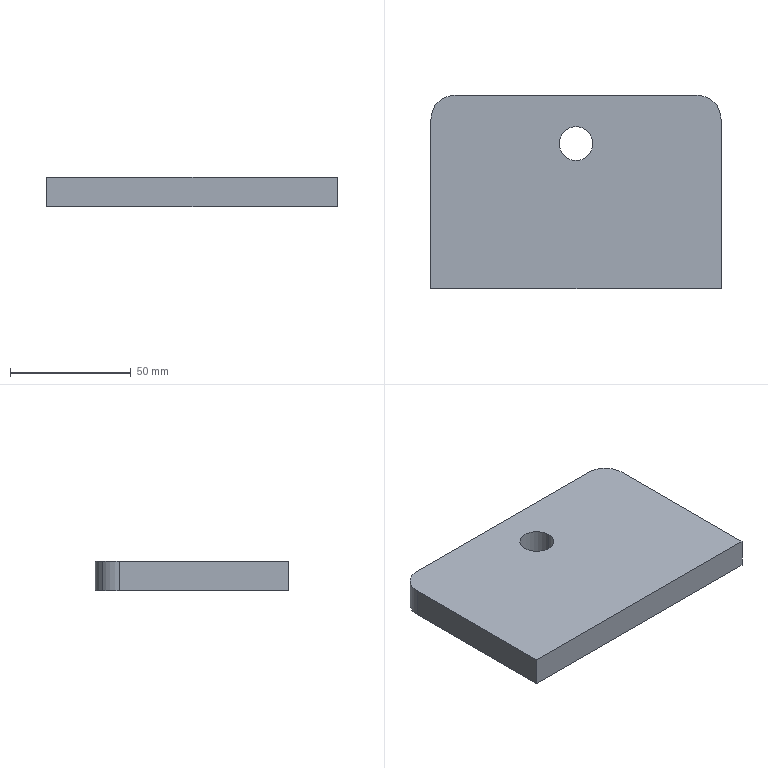Part | STEP file | DCV-000-022 | 1 solid | 12 faces | box 120 x 80 x 12 mm | volume 112838 mm3 | cylinder 6 | plane 6 | commonest cylinder face diameters 20 x4 14 x2
STEP:
#1=CARTESIAN_POINT('',(0.,0.,0.));
#2=DIRECTION('',(0.,0.,1.));
#3=DIRECTION('',(1.,0.,0.));
#4=AXIS2_PLACEMENT_3D('',#1,#2,#3);
#5=CARTESIAN_POINT('',(60.,70.,0.));
#6=VERTEX_POINT('',#5);
#7=CARTESIAN_POINT('',(57.071,77.071,0.));
#8=VERTEX_POINT('',#7);
#9=CARTESIAN_POINT('',(50.,70.,0.));
#10=DIRECTION('',(0.,0.,1.));
#11=DIRECTION('',(0.7071,0.7071,0.));
#12=AXIS2_PLACEMENT_3D('',#9,#10,#11);
#13=CIRCLE('',#12,10.);
#14=CARTESIAN_POINT('',(50.,70.,0.));
#15=DIRECTION('',(0.,0.,1.));
#16=DIRECTION('',(0.7071,0.7071,0.));
#17=AXIS2_PLACEMENT_3D('',#14,#15,#16);
#18=CYLINDRICAL_SURFACE('',#17,10.);
#19=CARTESIAN_POINT('',(0.,0.));
#20=DIRECTION('',(1.,0.));
#21=VECTOR('',#20,1.);
#22=LINE('',#19,#21);
#23=(GEOMETRIC_REPRESENTATION_CONTEXT(2)PARAMETRIC_REPRESENTATION_CONTEXT()REPRESENTATION_CONTEXT('',''));
#24=DEFINITIONAL_REPRESENTATION('',(#22),#23);
#25=PCURVE('',#18,#24);
#26=CARTESIAN_POINT('',(-0.000004309,40.,0.));
#27=DIRECTION('',(0.,0.,1.));
#28=DIRECTION('',(1.,0.,0.));
#29=AXIS2_PLACEMENT_3D('',#26,#27,#28);
#30=PLANE('',#29);
#31=CARTESIAN_POINT('',(50.,30.));
#32=DIRECTION('',(0.7071,0.7071));
#33=AXIS2_PLACEMENT_2D('',#31,#32);
#34=CIRCLE('',#33,10.);
#35=(GEOMETRIC_REPRESENTATION_CONTEXT(2)PARAMETRIC_REPRESENTATION_CONTEXT()REPRESENTATION_CONTEXT('',''));
#36=DEFINITIONAL_REPRESENTATION('',(#34),#35);
#37=PCURVE('',#30,#36);
#38=SURFACE_CURVE('',#13,(#25,#37),.PCURVE_S1.);
#39=EDGE_CURVE('',#6,#8,#38,.T.);
#40=ORIENTED_EDGE('',*,*,#39,.T.);
#41=CARTESIAN_POINT('',(57.071,77.071,12.));
#42=VERTEX_POINT('',#41);
#43=CARTESIAN_POINT('',(57.071,77.071,0.));
#44=DIRECTION('',(0.,0.,1.));
#45=VECTOR('',#44,1.);
#46=LINE('',#43,#45);
#47=CARTESIAN_POINT('',(6.283,0.));
#48=DIRECTION('',(0.,1.));
#49=VECTOR('',#48,1.);
#50=LINE('',#47,#49);
#51=(GEOMETRIC_REPRESENTATION_CONTEXT(2)PARAMETRIC_REPRESENTATION_CONTEXT()REPRESENTATION_CONTEXT('',''));
#52=DEFINITIONAL_REPRESENTATION('',(#50),#51);
#53=PCURVE('',#18,#52);
#54=CARTESIAN_POINT('',(50.,70.,0.));
#55=DIRECTION('',(0.,0.,1.));
#56=DIRECTION('',(0.7071,0.7071,0.));
#57=AXIS2_PLACEMENT_3D('',#54,#55,#56);
#58=CYLINDRICAL_SURFACE('',#57,10.);
#59=CARTESIAN_POINT('',(0.,0.));
#60=DIRECTION('',(0.,1.));
#61=VECTOR('',#60,1.);
#62=LINE('',#59,#61);
#63=(GEOMETRIC_REPRESENTATION_CONTEXT(2)PARAMETRIC_REPRESENTATION_CONTEXT()REPRESENTATION_CONTEXT('',''));
#64=DEFINITIONAL_REPRESENTATION('',(#62),#63);
#65=PCURVE('',#58,#64);
#66=SURFACE_CURVE('',#46,(#53,#65),.PCURVE_S1.);
#67=EDGE_CURVE('',#8,#42,#66,.T.);
#68=ORIENTED_EDGE('',*,*,#67,.T.);
#69=CARTESIAN_POINT('',(60.,70.,12.));
#70=VERTEX_POINT('',#69);
#71=CARTESIAN_POINT('',(50.,70.,12.));
#72=DIRECTION('',(0.,0.,-1.));
#73=DIRECTION('',(0.7071,0.7071,0.));
#74=AXIS2_PLACEMENT_3D('',#71,#72,#73);
#75=CIRCLE('',#74,10.);
#76=CARTESIAN_POINT('',(6.283,12.));
#77=DIRECTION('',(-1.,0.));
#78=VECTOR('',#77,1.);
#79=LINE('',#76,#78);
#80=(GEOMETRIC_REPRESENTATION_CONTEXT(2)PARAMETRIC_REPRESENTATION_CONTEXT()REPRESENTATION_CONTEXT('',''));
#81=DEFINITIONAL_REPRESENTATION('',(#79),#80);
#82=PCURVE('',#18,#81);
#83=CARTESIAN_POINT('',(-0.000004309,40.,12.));
#84=DIRECTION('',(0.,0.,1.));
#85=DIRECTION('',(1.,0.,0.));
#86=AXIS2_PLACEMENT_3D('',#83,#84,#85);
#87=PLANE('',#86);
#88=CARTESIAN_POINT('',(57.071,37.071));
#89=CARTESIAN_POINT('',(69.319,24.824));
#90=CARTESIAN_POINT('',(52.588,20.341));
#91=CARTESIAN_POINT('',(35.858,15.858));
#92=CARTESIAN_POINT('',(40.341,32.588));
#93=CARTESIAN_POINT('',(44.824,49.318));
#94=CARTESIAN_POINT('',(57.071,37.071));
#95=(BOUNDED_CURVE()B_SPLINE_CURVE(2,(#88,#89,#90,#91,#92,#93,#94),.UNSPECIFIED.,.T.,.F.)B_SPLINE_CURVE_WITH_KNOTS((1,2,2,2,2,1),(-2.094,0.,2.094,4.189,6.283,8.378),.UNSPECIFIED.)CURVE()GEOMETRIC_REPRESENTATION_ITEM()RATIONAL_B_SPLINE_CURVE((1.,0.5,1.,0.5,1.,0.5,1.))REPRESENTATION_ITEM(''));
#96=(GEOMETRIC_REPRESENTATION_CONTEXT(2)PARAMETRIC_REPRESENTATION_CONTEXT()REPRESENTATION_CONTEXT('',''));
#97=DEFINITIONAL_REPRESENTATION('',(#95),#96);
#98=PCURVE('',#87,#97);
#99=SURFACE_CURVE('',#75,(#82,#98),.PCURVE_S1.);
#100=EDGE_CURVE('',#42,#70,#99,.T.);
#101=ORIENTED_EDGE('',*,*,#100,.T.);
#102=CARTESIAN_POINT('',(60.,70.,0.));
#103=DIRECTION('',(0.,0.,-1.));
#104=VECTOR('',#103,1.);
#105=LINE('',#102,#104);
#106=CARTESIAN_POINT('',(5.498,0.));
#107=DIRECTION('',(0.,-1.));
#108=VECTOR('',#107,1.);
#109=LINE('',#106,#108);
#110=(GEOMETRIC_REPRESENTATION_CONTEXT(2)PARAMETRIC_REPRESENTATION_CONTEXT()REPRESENTATION_CONTEXT('',''));
#111=DEFINITIONAL_REPRESENTATION('',(#109),#110);
#112=PCURVE('',#18,#111);
#113=CARTESIAN_POINT('',(60.,-0.000000612,0.));
#114=DIRECTION('',(1.,-0.000000215,0.));
#115=DIRECTION('',(0.,0.,-1.));
#116=AXIS2_PLACEMENT_3D('',#113,#114,#115);
#117=PLANE('',#116);
#118=CARTESIAN_POINT('',(0.,70.));
#119=DIRECTION('',(1.,0.));
#120=VECTOR('',#119,1.);
#121=LINE('',#118,#120);
#122=(GEOMETRIC_REPRESENTATION_CONTEXT(2)PARAMETRIC_REPRESENTATION_CONTEXT()REPRESENTATION_CONTEXT('',''));
#123=DEFINITIONAL_REPRESENTATION('',(#121),#122);
#124=PCURVE('',#117,#123);
#125=SURFACE_CURVE('',#105,(#112,#124),.PCURVE_S1.);
#126=EDGE_CURVE('',#70,#6,#125,.T.);
#127=ORIENTED_EDGE('',*,*,#126,.T.);
#128=EDGE_LOOP('',(#40,#68,#101,#127));
#129=FACE_BOUND('',#128,.T.);
#130=ADVANCED_FACE('',(#129),#18,.T.);
#131=CARTESIAN_POINT('',(-50.,80.,0.));
#132=VERTEX_POINT('',#131);
#133=CARTESIAN_POINT('',(-57.071,77.071,0.));
#134=VERTEX_POINT('',#133);
#135=CARTESIAN_POINT('',(-50.,70.,0.));
#136=DIRECTION('',(0.,0.,1.));
#137=DIRECTION('',(-0.7071,0.7071,0.));
#138=AXIS2_PLACEMENT_3D('',#135,#136,#137);
#139=CIRCLE('',#138,10.);
#140=CARTESIAN_POINT('',(-50.,70.,0.));
#141=DIRECTION('',(0.,0.,1.));
#142=DIRECTION('',(-0.7071,0.7071,0.));
#143=AXIS2_PLACEMENT_3D('',#140,#141,#142);
#144=CYLINDRICAL_SURFACE('',#143,10.);
#145=CARTESIAN_POINT('',(0.,0.));
#146=DIRECTION('',(1.,0.));
#147=VECTOR('',#146,1.);
#148=LINE('',#145,#147);
#149=(GEOMETRIC_REPRESENTATION_CONTEXT(2)PARAMETRIC_REPRESENTATION_CONTEXT()REPRESENTATION_CONTEXT('',''));
#150=DEFINITIONAL_REPRESENTATION('',(#148),#149);
#151=PCURVE('',#144,#150);
#152=CARTESIAN_POINT('',(-50.,30.));
#153=DIRECTION('',(-0.7071,0.7071));
#154=AXIS2_PLACEMENT_2D('',#152,#153);
#155=CIRCLE('',#154,10.);
#156=(GEOMETRIC_REPRESENTATION_CONTEXT(2)PARAMETRIC_REPRESENTATION_CONTEXT()REPRESENTATION_CONTEXT('',''));
#157=DEFINITIONAL_REPRESENTATION('',(#155),#156);
#158=PCURVE('',#30,#157);
#159=SURFACE_CURVE('',#139,(#151,#158),.PCURVE_S1.);
#160=EDGE_CURVE('',#132,#134,#159,.T.);
#161=ORIENTED_EDGE('',*,*,#160,.T.);
#162=CARTESIAN_POINT('',(-57.071,77.071,12.));
#163=VERTEX_POINT('',#162);
#164=CARTESIAN_POINT('',(-57.071,77.071,0.));
#165=DIRECTION('',(0.,0.,1.));
#166=VECTOR('',#165,1.);
#167=LINE('',#164,#166);
#168=CARTESIAN_POINT('',(6.283,0.));
#169=DIRECTION('',(0.,1.));
#170=VECTOR('',#169,1.);
#171=LINE('',#168,#170);
#172=(GEOMETRIC_REPRESENTATION_CONTEXT(2)PARAMETRIC_REPRESENTATION_CONTEXT()REPRESENTATION_CONTEXT('',''));
#173=DEFINITIONAL_REPRESENTATION('',(#171),#172);
#174=PCURVE('',#144,#173);
#175=CARTESIAN_POINT('',(-50.,70.,0.));
#176=DIRECTION('',(0.,0.,1.));
#177=DIRECTION('',(-0.7071,0.7071,0.));
#178=AXIS2_PLACEMENT_3D('',#175,#176,#177);
#179=CYLINDRICAL_SURFACE('',#178,10.);
#180=CARTESIAN_POINT('',(0.,0.));
#181=DIRECTION('',(0.,1.));
#182=VECTOR('',#181,1.);
#183=LINE('',#180,#182);
#184=(GEOMETRIC_REPRESENTATION_CONTEXT(2)PARAMETRIC_REPRESENTATION_CONTEXT()REPRESENTATION_CONTEXT('',''));
#185=DEFINITIONAL_REPRESENTATION('',(#183),#184);
#186=PCURVE('',#179,#185);
#187=SURFACE_CURVE('',#167,(#174,#186),.PCURVE_S1.);
#188=EDGE_CURVE('',#134,#163,#187,.T.);
#189=ORIENTED_EDGE('',*,*,#188,.T.);
#190=CARTESIAN_POINT('',(-50.,80.,12.));
#191=VERTEX_POINT('',#190);
#192=CARTESIAN_POINT('',(-50.,70.,12.));
#193=DIRECTION('',(0.,0.,-1.));
#194=DIRECTION('',(-0.7071,0.7071,0.));
#195=AXIS2_PLACEMENT_3D('',#192,#193,#194);
#196=CIRCLE('',#195,10.);
#197=CARTESIAN_POINT('',(6.283,12.));
#198=DIRECTION('',(-1.,0.));
#199=VECTOR('',#198,1.);
#200=LINE('',#197,#199);
#201=(GEOMETRIC_REPRESENTATION_CONTEXT(2)PARAMETRIC_REPRESENTATION_CONTEXT()REPRESENTATION_CONTEXT('',''));
#202=DEFINITIONAL_REPRESENTATION('',(#200),#201);
#203=PCURVE('',#144,#202);
#204=CARTESIAN_POINT('',(-57.071,37.071));
#205=CARTESIAN_POINT('',(-44.824,49.319));
#206=CARTESIAN_POINT('',(-40.341,32.588));
#207=CARTESIAN_POINT('',(-35.858,15.858));
#208=CARTESIAN_POINT('',(-52.588,20.341));
#209=CARTESIAN_POINT('',(-69.319,24.824));
#210=CARTESIAN_POINT('',(-57.071,37.071));
#211=(BOUNDED_CURVE()B_SPLINE_CURVE(2,(#204,#205,#206,#207,#208,#209,#210),.UNSPECIFIED.,.T.,.F.)B_SPLINE_CURVE_WITH_KNOTS((1,2,2,2,2,1),(-2.094,0.,2.094,4.189,6.283,8.378),.UNSPECIFIED.)CURVE()GEOMETRIC_REPRESENTATION_ITEM()RATIONAL_B_SPLINE_CURVE((1.,0.5,1.,0.5,1.,0.5,1.))REPRESENTATION_ITEM(''));
#212=(GEOMETRIC_REPRESENTATION_CONTEXT(2)PARAMETRIC_REPRESENTATION_CONTEXT()REPRESENTATION_CONTEXT('',''));
#213=DEFINITIONAL_REPRESENTATION('',(#211),#212);
#214=PCURVE('',#87,#213);
#215=SURFACE_CURVE('',#196,(#203,#214),.PCURVE_S1.);
#216=EDGE_CURVE('',#163,#191,#215,.T.);
#217=ORIENTED_EDGE('',*,*,#216,.T.);
#218=CARTESIAN_POINT('',(-50.,80.,0.));
#219=DIRECTION('',(0.,0.,-1.));
#220=VECTOR('',#219,1.);
#221=LINE('',#218,#220);
#222=CARTESIAN_POINT('',(5.498,0.));
#223=DIRECTION('',(0.,-1.));
#224=VECTOR('',#223,1.);
#225=LINE('',#222,#224);
#226=(GEOMETRIC_REPRESENTATION_CONTEXT(2)PARAMETRIC_REPRESENTATION_CONTEXT()REPRESENTATION_CONTEXT('',''));
#227=DEFINITIONAL_REPRESENTATION('',(#225),#226);
#228=PCURVE('',#144,#227);
#229=CARTESIAN_POINT('',(60.,80.,0.));
#230=DIRECTION('',(0.000000215,1.,0.));
#231=DIRECTION('',(0.,0.,-1.));
#232=AXIS2_PLACEMENT_3D('',#229,#230,#231);
#233=PLANE('',#232);
#234=CARTESIAN_POINT('',(0.,110.));
#235=DIRECTION('',(1.,0.));
#236=VECTOR('',#235,1.);
#237=LINE('',#234,#236);
#238=(GEOMETRIC_REPRESENTATION_CONTEXT(2)PARAMETRIC_REPRESENTATION_CONTEXT()REPRESENTATION_CONTEXT('',''));
#239=DEFINITIONAL_REPRESENTATION('',(#237),#238);
#240=PCURVE('',#233,#239);
#241=SURFACE_CURVE('',#221,(#228,#240),.PCURVE_S1.);
#242=EDGE_CURVE('',#191,#132,#241,.T.);
#243=ORIENTED_EDGE('',*,*,#242,.T.);
#244=EDGE_LOOP('',(#161,#189,#217,#243));
#245=FACE_BOUND('',#244,.T.);
#246=ADVANCED_FACE('',(#245),#144,.T.);
#247=CARTESIAN_POINT('',(7.,60.,0.));
#248=VERTEX_POINT('',#247);
#249=CARTESIAN_POINT('',(7.,60.,12.));
#250=VERTEX_POINT('',#249);
#251=CARTESIAN_POINT('',(7.,60.,144.72));
#252=DIRECTION('',(0.,0.,1.));
#253=VECTOR('',#252,1.);
#254=LINE('',#251,#253);
#255=CARTESIAN_POINT('',(0.,60.,144.72));
#256=DIRECTION('',(0.,0.,1.));
#257=DIRECTION('',(1.,0.,0.));
#258=AXIS2_PLACEMENT_3D('',#255,#256,#257);
#259=CYLINDRICAL_SURFACE('',#258,7.);
#260=CARTESIAN_POINT('',(6.283,0.));
#261=DIRECTION('',(0.,1.));
#262=VECTOR('',#261,1.);
#263=LINE('',#260,#262);
#264=(GEOMETRIC_REPRESENTATION_CONTEXT(2)PARAMETRIC_REPRESENTATION_CONTEXT()REPRESENTATION_CONTEXT('',''));
#265=DEFINITIONAL_REPRESENTATION('',(#263),#264);
#266=PCURVE('',#259,#265);
#267=CARTESIAN_POINT('',(0.,60.,144.72));
#268=DIRECTION('',(0.,0.,1.));
#269=DIRECTION('',(1.,0.,0.));
#270=AXIS2_PLACEMENT_3D('',#267,#268,#269);
#271=CYLINDRICAL_SURFACE('',#270,7.);
#272=CARTESIAN_POINT('',(0.,0.));
#273=DIRECTION('',(0.,1.));
#274=VECTOR('',#273,1.);
#275=LINE('',#272,#274);
#276=(GEOMETRIC_REPRESENTATION_CONTEXT(2)PARAMETRIC_REPRESENTATION_CONTEXT()REPRESENTATION_CONTEXT('',''));
#277=DEFINITIONAL_REPRESENTATION('',(#275),#276);
#278=PCURVE('',#271,#277);
#279=SURFACE_CURVE('',#254,(#266,#278),.PCURVE_S1.);
#280=EDGE_CURVE('',#248,#250,#279,.T.);
#281=ORIENTED_EDGE('',*,*,#280,.T.);
#282=CARTESIAN_POINT('',(-7.,60.,12.));
#283=VERTEX_POINT('',#282);
#284=CARTESIAN_POINT('',(0.,60.,12.));
#285=DIRECTION('',(0.,0.,-1.));
#286=DIRECTION('',(1.,0.,0.));
#287=AXIS2_PLACEMENT_3D('',#284,#285,#286);
#288=CIRCLE('',#287,7.);
#289=CARTESIAN_POINT('',(6.283,-132.72));
#290=DIRECTION('',(-1.,0.));
#291=VECTOR('',#290,1.);
#292=LINE('',#289,#291);
#293=(GEOMETRIC_REPRESENTATION_CONTEXT(2)PARAMETRIC_REPRESENTATION_CONTEXT()REPRESENTATION_CONTEXT('',''));
#294=DEFINITIONAL_REPRESENTATION('',(#292),#293);
#295=PCURVE('',#259,#294);
#296=CARTESIAN_POINT('',(7.,20.));
#297=CARTESIAN_POINT('',(7.,7.876));
#298=CARTESIAN_POINT('',(-3.5,13.938));
#299=CARTESIAN_POINT('',(-14.,20.));
#300=CARTESIAN_POINT('',(-3.5,26.062));
#301=CARTESIAN_POINT('',(7.,32.124));
#302=CARTESIAN_POINT('',(7.,20.));
#303=(BOUNDED_CURVE()B_SPLINE_CURVE(2,(#296,#297,#298,#299,#300,#301,#302),.UNSPECIFIED.,.T.,.F.)B_SPLINE_CURVE_WITH_KNOTS((1,2,2,2,2,1),(-2.094,0.,2.094,4.189,6.283,8.378),.UNSPECIFIED.)CURVE()GEOMETRIC_REPRESENTATION_ITEM()RATIONAL_B_SPLINE_CURVE((1.,0.5,1.,0.5,1.,0.5,1.))REPRESENTATION_ITEM(''));
#304=(GEOMETRIC_REPRESENTATION_CONTEXT(2)PARAMETRIC_REPRESENTATION_CONTEXT()REPRESENTATION_CONTEXT('',''));
#305=DEFINITIONAL_REPRESENTATION('',(#303),#304);
#306=PCURVE('',#87,#305);
#307=SURFACE_CURVE('',#288,(#295,#306),.PCURVE_S1.);
#308=EDGE_CURVE('',#250,#283,#307,.T.);
#309=ORIENTED_EDGE('',*,*,#308,.T.);
#310=CARTESIAN_POINT('',(-7.,60.,0.));
#311=VERTEX_POINT('',#310);
#312=CARTESIAN_POINT('',(-7.,60.,144.72));
#313=DIRECTION('',(0.,0.,1.));
#314=VECTOR('',#313,1.);
#315=LINE('',#312,#314);
#316=CARTESIAN_POINT('',(3.142,0.));
#317=DIRECTION('',(0.,1.));
#318=VECTOR('',#317,1.);
#319=LINE('',#316,#318);
#320=(GEOMETRIC_REPRESENTATION_CONTEXT(2)PARAMETRIC_REPRESENTATION_CONTEXT()REPRESENTATION_CONTEXT('',''));
#321=DEFINITIONAL_REPRESENTATION('',(#319),#320);
#322=PCURVE('',#259,#321);
#323=CARTESIAN_POINT('',(3.142,0.));
#324=DIRECTION('',(0.,1.));
#325=VECTOR('',#324,1.);
#326=LINE('',#323,#325);
#327=(GEOMETRIC_REPRESENTATION_CONTEXT(2)PARAMETRIC_REPRESENTATION_CONTEXT()REPRESENTATION_CONTEXT('',''));
#328=DEFINITIONAL_REPRESENTATION('',(#326),#327);
#329=PCURVE('',#271,#328);
#330=SURFACE_CURVE('',#315,(#322,#329),.PCURVE_S1.);
#331=EDGE_CURVE('',#311,#283,#330,.T.);
#332=ORIENTED_EDGE('',*,*,#331,.F.);
#333=CARTESIAN_POINT('',(0.,60.,0.));
#334=DIRECTION('',(0.,0.,1.));
#335=DIRECTION('',(1.,0.,0.));
#336=AXIS2_PLACEMENT_3D('',#333,#334,#335);
#337=CIRCLE('',#336,7.);
#338=CARTESIAN_POINT('',(0.,-144.72));
#339=DIRECTION('',(1.,0.));
#340=VECTOR('',#339,1.);
#341=LINE('',#338,#340);
#342=(GEOMETRIC_REPRESENTATION_CONTEXT(2)PARAMETRIC_REPRESENTATION_CONTEXT()REPRESENTATION_CONTEXT('',''));
#343=DEFINITIONAL_REPRESENTATION('',(#341),#342);
#344=PCURVE('',#259,#343);
#345=CARTESIAN_POINT('',(0.000004309,20.));
#346=DIRECTION('',(1.,0.));
#347=AXIS2_PLACEMENT_2D('',#345,#346);
#348=CIRCLE('',#347,7.);
#349=(GEOMETRIC_REPRESENTATION_CONTEXT(2)PARAMETRIC_REPRESENTATION_CONTEXT()REPRESENTATION_CONTEXT('',''));
#350=DEFINITIONAL_REPRESENTATION('',(#348),#349);
#351=PCURVE('',#30,#350);
#352=SURFACE_CURVE('',#337,(#344,#351),.PCURVE_S1.);
#353=EDGE_CURVE('',#311,#248,#352,.T.);
#354=ORIENTED_EDGE('',*,*,#353,.T.);
#355=EDGE_LOOP('',(#281,#309,#332,#354));
#356=FACE_BOUND('',#355,.F.);
#357=ADVANCED_FACE('',(#356),#259,.F.);
#358=ORIENTED_EDGE('',*,*,#308,.T.);
#359=CARTESIAN_POINT('',(0.,60.,12.));
#360=DIRECTION('',(0.,0.,-1.));
#361=DIRECTION('',(1.,0.,0.));
#362=AXIS2_PLACEMENT_3D('',#359,#360,#361);
#363=CIRCLE('',#362,7.);
#364=CARTESIAN_POINT('',(7.,20.));
#365=CARTESIAN_POINT('',(7.,7.876));
#366=CARTESIAN_POINT('',(-3.5,13.938));
#367=CARTESIAN_POINT('',(-14.,20.));
#368=CARTESIAN_POINT('',(-3.5,26.062));
#369=CARTESIAN_POINT('',(7.,32.124));
#370=CARTESIAN_POINT('',(7.,20.));
#371=(BOUNDED_CURVE()B_SPLINE_CURVE(2,(#364,#365,#366,#367,#368,#369,#370),.UNSPECIFIED.,.T.,.F.)B_SPLINE_CURVE_WITH_KNOTS((1,2,2,2,2,1),(-2.094,0.,2.094,4.189,6.283,8.378),.UNSPECIFIED.)CURVE()GEOMETRIC_REPRESENTATION_ITEM()RATIONAL_B_SPLINE_CURVE((1.,0.5,1.,0.5,1.,0.5,1.))REPRESENTATION_ITEM(''));
#372=(GEOMETRIC_REPRESENTATION_CONTEXT(2)PARAMETRIC_REPRESENTATION_CONTEXT()REPRESENTATION_CONTEXT('',''));
#373=DEFINITIONAL_REPRESENTATION('',(#371),#372);
#374=PCURVE('',#87,#373);
#375=CARTESIAN_POINT('',(6.283,-132.72));
#376=DIRECTION('',(-1.,0.));
#377=VECTOR('',#376,1.);
#378=LINE('',#375,#377);
#379=(GEOMETRIC_REPRESENTATION_CONTEXT(2)PARAMETRIC_REPRESENTATION_CONTEXT()REPRESENTATION_CONTEXT('',''));
#380=DEFINITIONAL_REPRESENTATION('',(#378),#379);
#381=PCURVE('',#271,#380);
#382=SURFACE_CURVE('',#363,(#374,#381),.PCURVE_S1.);
#383=EDGE_CURVE('',#283,#250,#382,.T.);
#384=ORIENTED_EDGE('',*,*,#383,.T.);
#385=EDGE_LOOP('',(#358,#384));
#386=FACE_BOUND('',#385,.T.);
#387=CARTESIAN_POINT('',(50.,80.,12.));
#388=VERTEX_POINT('',#387);
#389=CARTESIAN_POINT('',(50.,70.,12.));
#390=DIRECTION('',(0.,0.,-1.));
#391=DIRECTION('',(0.7071,0.7071,0.));
#392=AXIS2_PLACEMENT_3D('',#389,#390,#391);
#393=CIRCLE('',#392,10.);
#394=CARTESIAN_POINT('',(57.071,37.071));
#395=CARTESIAN_POINT('',(69.319,24.824));
#396=CARTESIAN_POINT('',(52.588,20.341));
#397=CARTESIAN_POINT('',(35.858,15.858));
#398=CARTESIAN_POINT('',(40.341,32.588));
#399=CARTESIAN_POINT('',(44.824,49.318));
#400=CARTESIAN_POINT('',(57.071,37.071));
#401=(BOUNDED_CURVE()B_SPLINE_CURVE(2,(#394,#395,#396,#397,#398,#399,#400),.UNSPECIFIED.,.T.,.F.)B_SPLINE_CURVE_WITH_KNOTS((1,2,2,2,2,1),(-2.094,0.,2.094,4.189,6.283,8.378),.UNSPECIFIED.)CURVE()GEOMETRIC_REPRESENTATION_ITEM()RATIONAL_B_SPLINE_CURVE((1.,0.5,1.,0.5,1.,0.5,1.))REPRESENTATION_ITEM(''));
#402=(GEOMETRIC_REPRESENTATION_CONTEXT(2)PARAMETRIC_REPRESENTATION_CONTEXT()REPRESENTATION_CONTEXT('',''));
#403=DEFINITIONAL_REPRESENTATION('',(#401),#402);
#404=PCURVE('',#87,#403);
#405=CARTESIAN_POINT('',(6.283,12.));
#406=DIRECTION('',(-1.,0.));
#407=VECTOR('',#406,1.);
#408=LINE('',#405,#407);
#409=(GEOMETRIC_REPRESENTATION_CONTEXT(2)PARAMETRIC_REPRESENTATION_CONTEXT()REPRESENTATION_CONTEXT('',''));
#410=DEFINITIONAL_REPRESENTATION('',(#408),#409);
#411=PCURVE('',#58,#410);
#412=SURFACE_CURVE('',#393,(#404,#411),.PCURVE_S1.);
#413=EDGE_CURVE('',#388,#42,#412,.T.);
#414=ORIENTED_EDGE('',*,*,#413,.F.);
#415=CARTESIAN_POINT('',(60.,80.,12.));
#416=DIRECTION('',(-1.,0.000000215,0.));
#417=VECTOR('',#416,1.);
#418=LINE('',#415,#417);
#419=CARTESIAN_POINT('',(60.,40.));
#420=DIRECTION('',(-1.,0.000000215));
#421=VECTOR('',#420,1.);
#422=LINE('',#419,#421);
#423=(GEOMETRIC_REPRESENTATION_CONTEXT(2)PARAMETRIC_REPRESENTATION_CONTEXT()REPRESENTATION_CONTEXT('',''));
#424=DEFINITIONAL_REPRESENTATION('',(#422),#423);
#425=PCURVE('',#87,#424);
#426=CARTESIAN_POINT('',(-12.,0.));
#427=DIRECTION('',(0.,1.));
#428=VECTOR('',#427,1.);
#429=LINE('',#426,#428);
#430=(GEOMETRIC_REPRESENTATION_CONTEXT(2)PARAMETRIC_REPRESENTATION_CONTEXT()REPRESENTATION_CONTEXT('',''));
#431=DEFINITIONAL_REPRESENTATION('',(#429),#430);
#432=PCURVE('',#233,#431);
#433=SURFACE_CURVE('',#418,(#425,#432),.PCURVE_S1.);
#434=EDGE_CURVE('',#388,#191,#433,.T.);
#435=ORIENTED_EDGE('',*,*,#434,.T.);
#436=ORIENTED_EDGE('',*,*,#216,.F.);
#437=CARTESIAN_POINT('',(-60.,70.,12.));
#438=VERTEX_POINT('',#437);
#439=CARTESIAN_POINT('',(-50.,70.,12.));
#440=DIRECTION('',(0.,0.,-1.));
#441=DIRECTION('',(-0.7071,0.7071,0.));
#442=AXIS2_PLACEMENT_3D('',#439,#440,#441);
#443=CIRCLE('',#442,10.);
#444=CARTESIAN_POINT('',(-57.071,37.071));
#445=CARTESIAN_POINT('',(-44.824,49.319));
#446=CARTESIAN_POINT('',(-40.341,32.588));
#447=CARTESIAN_POINT('',(-35.858,15.858));
#448=CARTESIAN_POINT('',(-52.588,20.341));
#449=CARTESIAN_POINT('',(-69.319,24.824));
#450=CARTESIAN_POINT('',(-57.071,37.071));
#451=(BOUNDED_CURVE()B_SPLINE_CURVE(2,(#444,#445,#446,#447,#448,#449,#450),.UNSPECIFIED.,.T.,.F.)B_SPLINE_CURVE_WITH_KNOTS((1,2,2,2,2,1),(-2.094,0.,2.094,4.189,6.283,8.378),.UNSPECIFIED.)CURVE()GEOMETRIC_REPRESENTATION_ITEM()RATIONAL_B_SPLINE_CURVE((1.,0.5,1.,0.5,1.,0.5,1.))REPRESENTATION_ITEM(''));
#452=(GEOMETRIC_REPRESENTATION_CONTEXT(2)PARAMETRIC_REPRESENTATION_CONTEXT()REPRESENTATION_CONTEXT('',''));
#453=DEFINITIONAL_REPRESENTATION('',(#451),#452);
#454=PCURVE('',#87,#453);
#455=CARTESIAN_POINT('',(6.283,12.));
#456=DIRECTION('',(-1.,0.));
#457=VECTOR('',#456,1.);
#458=LINE('',#455,#457);
#459=(GEOMETRIC_REPRESENTATION_CONTEXT(2)PARAMETRIC_REPRESENTATION_CONTEXT()REPRESENTATION_CONTEXT('',''));
#460=DEFINITIONAL_REPRESENTATION('',(#458),#459);
#461=PCURVE('',#179,#460);
#462=SURFACE_CURVE('',#443,(#454,#461),.PCURVE_S1.);
#463=EDGE_CURVE('',#438,#163,#462,.T.);
#464=ORIENTED_EDGE('',*,*,#463,.F.);
#465=CARTESIAN_POINT('',(-60.,0.000000612,12.));
#466=VERTEX_POINT('',#465);
#467=CARTESIAN_POINT('',(-60.,80.,12.));
#468=DIRECTION('',(-0.000000215,-1.,0.));
#469=VECTOR('',#468,1.);
#470=LINE('',#467,#469);
#471=CARTESIAN_POINT('',(-60.,40.));
#472=DIRECTION('',(-0.000000215,-1.));
#473=VECTOR('',#472,1.);
#474=LINE('',#471,#473);
#475=(GEOMETRIC_REPRESENTATION_CONTEXT(2)PARAMETRIC_REPRESENTATION_CONTEXT()REPRESENTATION_CONTEXT('',''));
#476=DEFINITIONAL_REPRESENTATION('',(#474),#475);
#477=PCURVE('',#87,#476);
#478=CARTESIAN_POINT('',(-60.,80.,0.));
#479=DIRECTION('',(-1.,0.000000215,0.));
#480=DIRECTION('',(0.,0.,1.));
#481=AXIS2_PLACEMENT_3D('',#478,#479,#480);
#482=PLANE('',#481);
#483=CARTESIAN_POINT('',(12.,0.));
#484=DIRECTION('',(0.,-1.));
#485=VECTOR('',#484,1.);
#486=LINE('',#483,#485);
#487=(GEOMETRIC_REPRESENTATION_CONTEXT(2)PARAMETRIC_REPRESENTATION_CONTEXT()REPRESENTATION_CONTEXT('',''));
#488=DEFINITIONAL_REPRESENTATION('',(#486),#487);
#489=PCURVE('',#482,#488);
#490=SURFACE_CURVE('',#470,(#477,#489),.PCURVE_S1.);
#491=EDGE_CURVE('',#438,#466,#490,.T.);
#492=ORIENTED_EDGE('',*,*,#491,.T.);
#493=CARTESIAN_POINT('',(60.,-0.000000612,12.));
#494=VERTEX_POINT('',#493);
#495=CARTESIAN_POINT('',(-60.,0.000000612,12.));
#496=DIRECTION('',(1.,-0.00000001,0.));
#497=VECTOR('',#496,1.);
#498=LINE('',#495,#497);
#499=CARTESIAN_POINT('',(-60.,-40.));
#500=DIRECTION('',(1.,-0.00000001));
#501=VECTOR('',#500,1.);
#502=LINE('',#499,#501);
#503=(GEOMETRIC_REPRESENTATION_CONTEXT(2)PARAMETRIC_REPRESENTATION_CONTEXT()REPRESENTATION_CONTEXT('',''));
#504=DEFINITIONAL_REPRESENTATION('',(#502),#503);
#505=PCURVE('',#87,#504);
#506=CARTESIAN_POINT('',(-60.,0.000000612,0.));
#507=DIRECTION('',(-0.00000001,-1.,0.));
#508=DIRECTION('',(-1.,0.00000001,0.));
#509=AXIS2_PLACEMENT_3D('',#506,#507,#508);
#510=PLANE('',#509);
#511=CARTESIAN_POINT('',(0.,-12.));
#512=DIRECTION('',(-1.,0.));
#513=VECTOR('',#512,1.);
#514=LINE('',#511,#513);
#515=(GEOMETRIC_REPRESENTATION_CONTEXT(2)PARAMETRIC_REPRESENTATION_CONTEXT()REPRESENTATION_CONTEXT('',''));
#516=DEFINITIONAL_REPRESENTATION('',(#514),#515);
#517=PCURVE('',#510,#516);
#518=SURFACE_CURVE('',#498,(#505,#517),.PCURVE_S1.);
#519=EDGE_CURVE('',#466,#494,#518,.T.);
#520=ORIENTED_EDGE('',*,*,#519,.T.);
#521=CARTESIAN_POINT('',(60.,-0.000000612,12.));
#522=DIRECTION('',(0.000000215,1.,0.));
#523=VECTOR('',#522,1.);
#524=LINE('',#521,#523);
#525=CARTESIAN_POINT('',(60.,-40.));
#526=DIRECTION('',(0.000000215,1.));
#527=VECTOR('',#526,1.);
#528=LINE('',#525,#527);
#529=(GEOMETRIC_REPRESENTATION_CONTEXT(2)PARAMETRIC_REPRESENTATION_CONTEXT()REPRESENTATION_CONTEXT('',''));
#530=DEFINITIONAL_REPRESENTATION('',(#528),#529);
#531=PCURVE('',#87,#530);
#532=CARTESIAN_POINT('',(-12.,0.));
#533=DIRECTION('',(0.,1.));
#534=VECTOR('',#533,1.);
#535=LINE('',#532,#534);
#536=(GEOMETRIC_REPRESENTATION_CONTEXT(2)PARAMETRIC_REPRESENTATION_CONTEXT()REPRESENTATION_CONTEXT('',''));
#537=DEFINITIONAL_REPRESENTATION('',(#535),#536);
#538=PCURVE('',#117,#537);
#539=SURFACE_CURVE('',#524,(#531,#538),.PCURVE_S1.);
#540=EDGE_CURVE('',#494,#70,#539,.T.);
#541=ORIENTED_EDGE('',*,*,#540,.T.);
#542=ORIENTED_EDGE('',*,*,#100,.F.);
#543=EDGE_LOOP('',(#414,#435,#436,#464,#492,#520,#541,#542));
#544=FACE_BOUND('',#543,.T.);
#545=ADVANCED_FACE('',(#386,#544),#87,.T.);
#546=CARTESIAN_POINT('',(-60.,70.,0.));
#547=VERTEX_POINT('',#546);
#548=CARTESIAN_POINT('',(-60.,70.,0.));
#549=DIRECTION('',(0.,0.,1.));
#550=VECTOR('',#549,1.);
#551=LINE('',#548,#550);
#552=CARTESIAN_POINT('',(0.,-10.));
#553=DIRECTION('',(1.,0.));
#554=VECTOR('',#553,1.);
#555=LINE('',#552,#554);
#556=(GEOMETRIC_REPRESENTATION_CONTEXT(2)PARAMETRIC_REPRESENTATION_CONTEXT()REPRESENTATION_CONTEXT('',''));
#557=DEFINITIONAL_REPRESENTATION('',(#555),#556);
#558=PCURVE('',#482,#557);
#559=CARTESIAN_POINT('',(0.7854,0.));
#560=DIRECTION('',(0.,1.));
#561=VECTOR('',#560,1.);
#562=LINE('',#559,#561);
#563=(GEOMETRIC_REPRESENTATION_CONTEXT(2)PARAMETRIC_REPRESENTATION_CONTEXT()REPRESENTATION_CONTEXT('',''));
#564=DEFINITIONAL_REPRESENTATION('',(#562),#563);
#565=PCURVE('',#179,#564);
#566=SURFACE_CURVE('',#551,(#558,#565),.PCURVE_S1.);
#567=EDGE_CURVE('',#547,#438,#566,.T.);
#568=ORIENTED_EDGE('',*,*,#567,.F.);
#569=CARTESIAN_POINT('',(-60.,0.000000612,0.));
#570=VERTEX_POINT('',#569);
#571=CARTESIAN_POINT('',(-60.,80.,0.));
#572=DIRECTION('',(-0.000000215,-1.,0.));
#573=VECTOR('',#572,1.);
#574=LINE('',#571,#573);
#575=CARTESIAN_POINT('',(0.,0.));
#576=DIRECTION('',(0.,-1.));
#577=VECTOR('',#576,1.);
#578=LINE('',#575,#577);
#579=(GEOMETRIC_REPRESENTATION_CONTEXT(2)PARAMETRIC_REPRESENTATION_CONTEXT()REPRESENTATION_CONTEXT('',''));
#580=DEFINITIONAL_REPRESENTATION('',(#578),#579);
#581=PCURVE('',#482,#580);
#582=CARTESIAN_POINT('',(-60.,40.));
#583=DIRECTION('',(-0.000000215,-1.));
#584=VECTOR('',#583,1.);
#585=LINE('',#582,#584);
#586=(GEOMETRIC_REPRESENTATION_CONTEXT(2)PARAMETRIC_REPRESENTATION_CONTEXT()REPRESENTATION_CONTEXT('',''));
#587=DEFINITIONAL_REPRESENTATION('',(#585),#586);
#588=PCURVE('',#30,#587);
#589=SURFACE_CURVE('',#574,(#581,#588),.PCURVE_S1.);
#590=EDGE_CURVE('',#547,#570,#589,.T.);
#591=ORIENTED_EDGE('',*,*,#590,.T.);
#592=CARTESIAN_POINT('',(-60.,0.000000612,0.));
#593=DIRECTION('',(0.,0.,1.));
#594=VECTOR('',#593,1.);
#595=LINE('',#592,#594);
#596=CARTESIAN_POINT('',(0.,-80.));
#597=DIRECTION('',(1.,0.));
#598=VECTOR('',#597,1.);
#599=LINE('',#596,#598);
#600=(GEOMETRIC_REPRESENTATION_CONTEXT(2)PARAMETRIC_REPRESENTATION_CONTEXT()REPRESENTATION_CONTEXT('',''));
#601=DEFINITIONAL_REPRESENTATION('',(#599),#600);
#602=PCURVE('',#482,#601);
#603=CARTESIAN_POINT('',(0.,0.));
#604=DIRECTION('',(0.,-1.));
#605=VECTOR('',#604,1.);
#606=LINE('',#603,#605);
#607=(GEOMETRIC_REPRESENTATION_CONTEXT(2)PARAMETRIC_REPRESENTATION_CONTEXT()REPRESENTATION_CONTEXT('',''));
#608=DEFINITIONAL_REPRESENTATION('',(#606),#607);
#609=PCURVE('',#510,#608);
#610=SURFACE_CURVE('',#595,(#602,#609),.PCURVE_S1.);
#611=EDGE_CURVE('',#570,#466,#610,.T.);
#612=ORIENTED_EDGE('',*,*,#611,.T.);
#613=ORIENTED_EDGE('',*,*,#491,.F.);
#614=EDGE_LOOP('',(#568,#591,#612,#613));
#615=FACE_BOUND('',#614,.T.);
#616=ADVANCED_FACE('',(#615),#482,.T.);
#617=CARTESIAN_POINT('',(60.,-0.000000612,0.));
#618=VERTEX_POINT('',#617);
#619=CARTESIAN_POINT('',(-60.,0.000000612,0.));
#620=DIRECTION('',(1.,-0.00000001,0.));
#621=VECTOR('',#620,1.);
#622=LINE('',#619,#621);
#623=CARTESIAN_POINT('',(0.,0.));
#624=DIRECTION('',(-1.,0.));
#625=VECTOR('',#624,1.);
#626=LINE('',#623,#625);
#627=(GEOMETRIC_REPRESENTATION_CONTEXT(2)PARAMETRIC_REPRESENTATION_CONTEXT()REPRESENTATION_CONTEXT('',''));
#628=DEFINITIONAL_REPRESENTATION('',(#626),#627);
#629=PCURVE('',#510,#628);
#630=CARTESIAN_POINT('',(-60.,-40.));
#631=DIRECTION('',(1.,-0.00000001));
#632=VECTOR('',#631,1.);
#633=LINE('',#630,#632);
#634=(GEOMETRIC_REPRESENTATION_CONTEXT(2)PARAMETRIC_REPRESENTATION_CONTEXT()REPRESENTATION_CONTEXT('',''));
#635=DEFINITIONAL_REPRESENTATION('',(#633),#634);
#636=PCURVE('',#30,#635);
#637=SURFACE_CURVE('',#622,(#629,#636),.PCURVE_S1.);
#638=EDGE_CURVE('',#570,#618,#637,.T.);
#639=ORIENTED_EDGE('',*,*,#638,.T.);
#640=CARTESIAN_POINT('',(60.,-0.000000612,0.));
#641=DIRECTION('',(0.,0.,1.));
#642=VECTOR('',#641,1.);
#643=LINE('',#640,#642);
#644=CARTESIAN_POINT('',(-120.,0.));
#645=DIRECTION('',(0.,-1.));
#646=VECTOR('',#645,1.);
#647=LINE('',#644,#646);
#648=(GEOMETRIC_REPRESENTATION_CONTEXT(2)PARAMETRIC_REPRESENTATION_CONTEXT()REPRESENTATION_CONTEXT('',''));
#649=DEFINITIONAL_REPRESENTATION('',(#647),#648);
#650=PCURVE('',#510,#649);
#651=CARTESIAN_POINT('',(0.,0.));
#652=DIRECTION('',(-1.,0.));
#653=VECTOR('',#652,1.);
#654=LINE('',#651,#653);
#655=(GEOMETRIC_REPRESENTATION_CONTEXT(2)PARAMETRIC_REPRESENTATION_CONTEXT()REPRESENTATION_CONTEXT('',''));
#656=DEFINITIONAL_REPRESENTATION('',(#654),#655);
#657=PCURVE('',#117,#656);
#658=SURFACE_CURVE('',#643,(#650,#657),.PCURVE_S1.);
#659=EDGE_CURVE('',#618,#494,#658,.T.);
#660=ORIENTED_EDGE('',*,*,#659,.T.);
#661=ORIENTED_EDGE('',*,*,#519,.F.);
#662=ORIENTED_EDGE('',*,*,#611,.F.);
#663=EDGE_LOOP('',(#639,#660,#661,#662));
#664=FACE_BOUND('',#663,.T.);
#665=ADVANCED_FACE('',(#664),#510,.T.);
#666=ORIENTED_EDGE('',*,*,#126,.F.);
#667=ORIENTED_EDGE('',*,*,#540,.F.);
#668=ORIENTED_EDGE('',*,*,#659,.F.);
#669=CARTESIAN_POINT('',(60.,-0.000000612,0.));
#670=DIRECTION('',(0.000000215,1.,0.));
#671=VECTOR('',#670,1.);
#672=LINE('',#669,#671);
#673=CARTESIAN_POINT('',(0.,0.));
#674=DIRECTION('',(0.,1.));
#675=VECTOR('',#674,1.);
#676=LINE('',#673,#675);
#677=(GEOMETRIC_REPRESENTATION_CONTEXT(2)PARAMETRIC_REPRESENTATION_CONTEXT()REPRESENTATION_CONTEXT('',''));
#678=DEFINITIONAL_REPRESENTATION('',(#676),#677);
#679=PCURVE('',#117,#678);
#680=CARTESIAN_POINT('',(60.,-40.));
#681=DIRECTION('',(0.000000215,1.));
#682=VECTOR('',#681,1.);
#683=LINE('',#680,#682);
#684=(GEOMETRIC_REPRESENTATION_CONTEXT(2)PARAMETRIC_REPRESENTATION_CONTEXT()REPRESENTATION_CONTEXT('',''));
#685=DEFINITIONAL_REPRESENTATION('',(#683),#684);
#686=PCURVE('',#30,#685);
#687=SURFACE_CURVE('',#672,(#679,#686),.PCURVE_S1.);
#688=EDGE_CURVE('',#618,#6,#687,.T.);
#689=ORIENTED_EDGE('',*,*,#688,.T.);
#690=EDGE_LOOP('',(#666,#667,#668,#689));
#691=FACE_BOUND('',#690,.T.);
#692=ADVANCED_FACE('',(#691),#117,.T.);
#693=ORIENTED_EDGE('',*,*,#383,.T.);
#694=ORIENTED_EDGE('',*,*,#280,.F.);
#695=CARTESIAN_POINT('',(0.,60.,0.));
#696=DIRECTION('',(0.,0.,1.));
#697=DIRECTION('',(1.,0.,0.));
#698=AXIS2_PLACEMENT_3D('',#695,#696,#697);
#699=CIRCLE('',#698,7.);
#700=CARTESIAN_POINT('',(0.,-144.72));
#701=DIRECTION('',(1.,0.));
#702=VECTOR('',#701,1.);
#703=LINE('',#700,#702);
#704=(GEOMETRIC_REPRESENTATION_CONTEXT(2)PARAMETRIC_REPRESENTATION_CONTEXT()REPRESENTATION_CONTEXT('',''));
#705=DEFINITIONAL_REPRESENTATION('',(#703),#704);
#706=PCURVE('',#271,#705);
#707=CARTESIAN_POINT('',(0.000004309,20.));
#708=DIRECTION('',(1.,0.));
#709=AXIS2_PLACEMENT_2D('',#707,#708);
#710=CIRCLE('',#709,7.);
#711=(GEOMETRIC_REPRESENTATION_CONTEXT(2)PARAMETRIC_REPRESENTATION_CONTEXT()REPRESENTATION_CONTEXT('',''));
#712=DEFINITIONAL_REPRESENTATION('',(#710),#711);
#713=PCURVE('',#30,#712);
#714=SURFACE_CURVE('',#699,(#706,#713),.PCURVE_S1.);
#715=EDGE_CURVE('',#248,#311,#714,.T.);
#716=ORIENTED_EDGE('',*,*,#715,.T.);
#717=ORIENTED_EDGE('',*,*,#331,.T.);
#718=EDGE_LOOP('',(#693,#694,#716,#717));
#719=FACE_BOUND('',#718,.F.);
#720=ADVANCED_FACE('',(#719),#271,.F.);
#721=ORIENTED_EDGE('',*,*,#188,.F.);
#722=CARTESIAN_POINT('',(-50.,70.,0.));
#723=DIRECTION('',(0.,0.,1.));
#724=DIRECTION('',(-0.7071,0.7071,0.));
#725=AXIS2_PLACEMENT_3D('',#722,#723,#724);
#726=CIRCLE('',#725,10.);
#727=CARTESIAN_POINT('',(0.,0.));
#728=DIRECTION('',(1.,0.));
#729=VECTOR('',#728,1.);
#730=LINE('',#727,#729);
#731=(GEOMETRIC_REPRESENTATION_CONTEXT(2)PARAMETRIC_REPRESENTATION_CONTEXT()REPRESENTATION_CONTEXT('',''));
#732=DEFINITIONAL_REPRESENTATION('',(#730),#731);
#733=PCURVE('',#179,#732);
#734=CARTESIAN_POINT('',(-50.,30.));
#735=DIRECTION('',(-0.7071,0.7071));
#736=AXIS2_PLACEMENT_2D('',#734,#735);
#737=CIRCLE('',#736,10.);
#738=(GEOMETRIC_REPRESENTATION_CONTEXT(2)PARAMETRIC_REPRESENTATION_CONTEXT()REPRESENTATION_CONTEXT('',''));
#739=DEFINITIONAL_REPRESENTATION('',(#737),#738);
#740=PCURVE('',#30,#739);
#741=SURFACE_CURVE('',#726,(#733,#740),.PCURVE_S1.);
#742=EDGE_CURVE('',#134,#547,#741,.T.);
#743=ORIENTED_EDGE('',*,*,#742,.T.);
#744=ORIENTED_EDGE('',*,*,#567,.T.);
#745=ORIENTED_EDGE('',*,*,#463,.T.);
#746=EDGE_LOOP('',(#721,#743,#744,#745));
#747=FACE_BOUND('',#746,.T.);
#748=ADVANCED_FACE('',(#747),#179,.T.);
#749=ORIENTED_EDGE('',*,*,#715,.T.);
#750=ORIENTED_EDGE('',*,*,#353,.T.);
#751=EDGE_LOOP('',(#749,#750));
#752=FACE_BOUND('',#751,.T.);
#753=ORIENTED_EDGE('',*,*,#39,.F.);
#754=ORIENTED_EDGE('',*,*,#688,.F.);
#755=ORIENTED_EDGE('',*,*,#638,.F.);
#756=ORIENTED_EDGE('',*,*,#590,.F.);
#757=ORIENTED_EDGE('',*,*,#742,.F.);
#758=ORIENTED_EDGE('',*,*,#160,.F.);
#759=CARTESIAN_POINT('',(50.,80.,0.));
#760=VERTEX_POINT('',#759);
#761=CARTESIAN_POINT('',(60.,80.,0.));
#762=DIRECTION('',(-1.,0.000000215,0.));
#763=VECTOR('',#762,1.);
#764=LINE('',#761,#763);
#765=CARTESIAN_POINT('',(60.,40.));
#766=DIRECTION('',(-1.,0.000000215));
#767=VECTOR('',#766,1.);
#768=LINE('',#765,#767);
#769=(GEOMETRIC_REPRESENTATION_CONTEXT(2)PARAMETRIC_REPRESENTATION_CONTEXT()REPRESENTATION_CONTEXT('',''));
#770=DEFINITIONAL_REPRESENTATION('',(#768),#769);
#771=PCURVE('',#30,#770);
#772=CARTESIAN_POINT('',(0.,0.));
#773=DIRECTION('',(0.,1.));
#774=VECTOR('',#773,1.);
#775=LINE('',#772,#774);
#776=(GEOMETRIC_REPRESENTATION_CONTEXT(2)PARAMETRIC_REPRESENTATION_CONTEXT()REPRESENTATION_CONTEXT('',''));
#777=DEFINITIONAL_REPRESENTATION('',(#775),#776);
#778=PCURVE('',#233,#777);
#779=SURFACE_CURVE('',#764,(#771,#778),.PCURVE_S1.);
#780=EDGE_CURVE('',#760,#132,#779,.T.);
#781=ORIENTED_EDGE('',*,*,#780,.F.);
#782=CARTESIAN_POINT('',(50.,70.,0.));
#783=DIRECTION('',(0.,0.,1.));
#784=DIRECTION('',(0.7071,0.7071,0.));
#785=AXIS2_PLACEMENT_3D('',#782,#783,#784);
#786=CIRCLE('',#785,10.);
#787=CARTESIAN_POINT('',(50.,30.));
#788=DIRECTION('',(0.7071,0.7071));
#789=AXIS2_PLACEMENT_2D('',#787,#788);
#790=CIRCLE('',#789,10.);
#791=(GEOMETRIC_REPRESENTATION_CONTEXT(2)PARAMETRIC_REPRESENTATION_CONTEXT()REPRESENTATION_CONTEXT('',''));
#792=DEFINITIONAL_REPRESENTATION('',(#790),#791);
#793=PCURVE('',#30,#792);
#794=CARTESIAN_POINT('',(0.,0.));
#795=DIRECTION('',(1.,0.));
#796=VECTOR('',#795,1.);
#797=LINE('',#794,#796);
#798=(GEOMETRIC_REPRESENTATION_CONTEXT(2)PARAMETRIC_REPRESENTATION_CONTEXT()REPRESENTATION_CONTEXT('',''));
#799=DEFINITIONAL_REPRESENTATION('',(#797),#798);
#800=PCURVE('',#58,#799);
#801=SURFACE_CURVE('',#786,(#793,#800),.PCURVE_S1.);
#802=EDGE_CURVE('',#8,#760,#801,.T.);
#803=ORIENTED_EDGE('',*,*,#802,.F.);
#804=EDGE_LOOP('',(#753,#754,#755,#756,#757,#758,#781,#803));
#805=FACE_BOUND('',#804,.T.);
#806=ADVANCED_FACE('',(#752,#805),#30,.F.);
#807=CARTESIAN_POINT('',(50.,80.,0.));
#808=DIRECTION('',(0.,0.,1.));
#809=VECTOR('',#808,1.);
#810=LINE('',#807,#809);
#811=CARTESIAN_POINT('',(0.,10.));
#812=DIRECTION('',(-1.,0.));
#813=VECTOR('',#812,1.);
#814=LINE('',#811,#813);
#815=(GEOMETRIC_REPRESENTATION_CONTEXT(2)PARAMETRIC_REPRESENTATION_CONTEXT()REPRESENTATION_CONTEXT('',''));
#816=DEFINITIONAL_REPRESENTATION('',(#814),#815);
#817=PCURVE('',#233,#816);
#818=CARTESIAN_POINT('',(0.7854,0.));
#819=DIRECTION('',(0.,1.));
#820=VECTOR('',#819,1.);
#821=LINE('',#818,#820);
#822=(GEOMETRIC_REPRESENTATION_CONTEXT(2)PARAMETRIC_REPRESENTATION_CONTEXT()REPRESENTATION_CONTEXT('',''));
#823=DEFINITIONAL_REPRESENTATION('',(#821),#822);
#824=PCURVE('',#58,#823);
#825=SURFACE_CURVE('',#810,(#817,#824),.PCURVE_S1.);
#826=EDGE_CURVE('',#760,#388,#825,.T.);
#827=ORIENTED_EDGE('',*,*,#826,.F.);
#828=ORIENTED_EDGE('',*,*,#780,.T.);
#829=ORIENTED_EDGE('',*,*,#242,.F.);
#830=ORIENTED_EDGE('',*,*,#434,.F.);
#831=EDGE_LOOP('',(#827,#828,#829,#830));
#832=FACE_BOUND('',#831,.T.);
#833=ADVANCED_FACE('',(#832),#233,.T.);
#834=ORIENTED_EDGE('',*,*,#67,.F.);
#835=ORIENTED_EDGE('',*,*,#802,.T.);
#836=ORIENTED_EDGE('',*,*,#826,.T.);
#837=ORIENTED_EDGE('',*,*,#413,.T.);
#838=EDGE_LOOP('',(#834,#835,#836,#837));
#839=FACE_BOUND('',#838,.T.);
#840=ADVANCED_FACE('',(#839),#58,.T.);
#841=CLOSED_SHELL('',(#130,#246,#357,#545,#616,#665,#692,#720,#748,#806,#833,#840));
#842=MANIFOLD_SOLID_BREP('',#841);
#843=(LENGTH_UNIT()NAMED_UNIT(*)SI_UNIT(.MILLI.,.METRE.));
#844=UNCERTAINTY_MEASURE_WITH_UNIT(LENGTH_MEASURE(0.0000001),#843,'','');
#845=(NAMED_UNIT(*)PLANE_ANGLE_UNIT()SI_UNIT($,.RADIAN.));
#846=(NAMED_UNIT(*)SI_UNIT($,.STERADIAN.)SOLID_ANGLE_UNIT());
#847=(GEOMETRIC_REPRESENTATION_CONTEXT(3)GLOBAL_UNCERTAINTY_ASSIGNED_CONTEXT((#844))GLOBAL_UNIT_ASSIGNED_CONTEXT((#843,#845,#846))REPRESENTATION_CONTEXT('',''));
#848=ADVANCED_BREP_SHAPE_REPRESENTATION('',(#4,#842),#847);